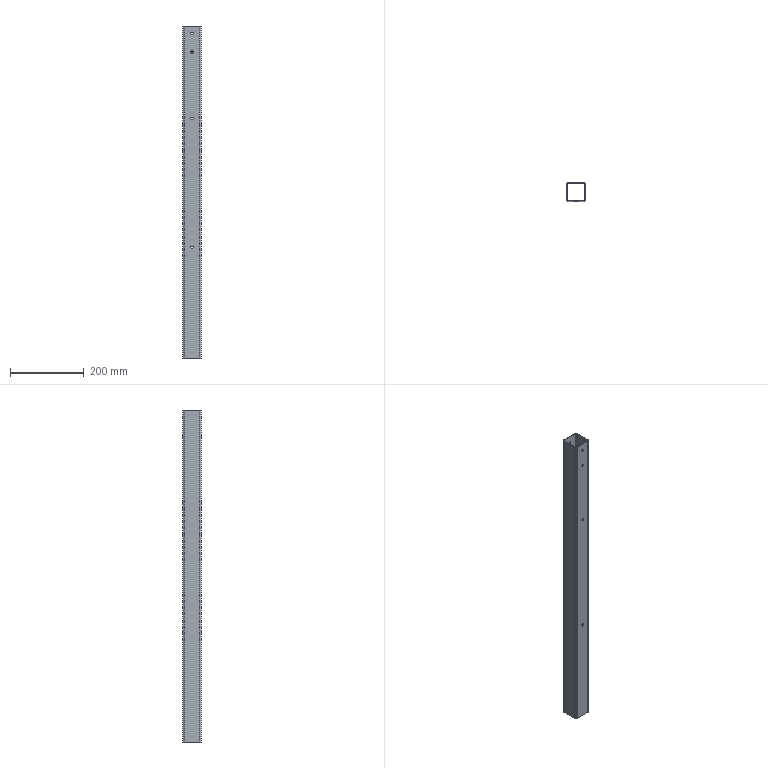Part | STEP file | 50x50xL-07 | 1 solid | 26 faces | box 50 x 50 x 900 mm | volume 334229 mm3 | plane 10 | spline 8 | cylinder 8 | commonest cylinder face diameters 5 x4 9 x4